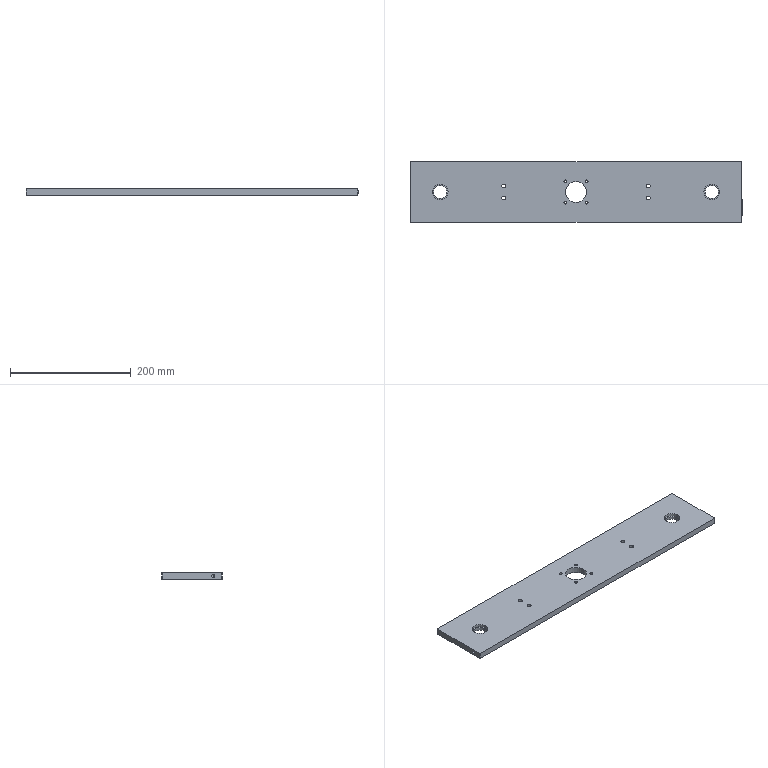Part | SolidWorks | features ICE 5, Extrusion 1, Fillet 1, HoleWzd 1, MirrorPattern 1 | 1 solid | 46 faces | box 550 x 100 x 10 mm | volume 528570 mm3 | cylinder 34 | plane 8 | cone 4 | commonest cylinder face diameters 4.5 x8 6.5 x8 2 x4 5 x4 22 x4 26 x4
STEP:
#1=CARTESIAN_POINT('',(257.,-35.,7.5));
#2=VERTEX_POINT('',#1);
#3=CARTESIAN_POINT('',(257.,-35.,2.5));
#4=VERTEX_POINT('',#3);
#5=CARTESIAN_POINT('',(257.,-35.,5.));
#6=DIRECTION('',(1.,0.,0.));
#7=DIRECTION('',(0.,0.,-1.));
#8=AXIS2_PLACEMENT_3D('',#5,#6,#7);
#9=CIRCLE('',#8,2.5);
#10=EDGE_CURVE('',#2,#4,#9,.T.);
#11=ORIENTED_EDGE('',*,*,#10,.F.);
#12=CARTESIAN_POINT('',(275.,-35.,7.5));
#13=VERTEX_POINT('',#12);
#14=CARTESIAN_POINT('',(275.,-35.,7.5));
#15=DIRECTION('',(1.,0.,0.));
#16=VECTOR('',#15,1000.);
#17=LINE('',#14,#16);
#18=EDGE_CURVE('',#2,#13,#17,.T.);
#19=ORIENTED_EDGE('',*,*,#18,.T.);
#20=CARTESIAN_POINT('',(275.,-35.,2.5));
#21=VERTEX_POINT('',#20);
#22=CARTESIAN_POINT('',(275.,-35.,5.));
#23=DIRECTION('',(1.,0.,0.));
#24=DIRECTION('',(0.,0.,-1.));
#25=AXIS2_PLACEMENT_3D('',#22,#23,#24);
#26=CIRCLE('',#25,2.5);
#27=EDGE_CURVE('',#13,#21,#26,.T.);
#28=ORIENTED_EDGE('',*,*,#27,.T.);
#29=CARTESIAN_POINT('',(275.,-35.,2.5));
#30=DIRECTION('',(1.,0.,0.));
#31=VECTOR('',#30,1000.);
#32=LINE('',#29,#31);
#33=EDGE_CURVE('',#4,#21,#32,.T.);
#34=ORIENTED_EDGE('',*,*,#33,.F.);
#35=EDGE_LOOP('',(#11,#19,#28,#34));
#36=FACE_OUTER_BOUND('',#35,.T.);
#37=CARTESIAN_POINT('',(275.,-35.,5.));
#38=DIRECTION('',(1.,0.,0.));
#39=DIRECTION('',(0.,0.,-1.));
#40=AXIS2_PLACEMENT_3D('',#37,#38,#39);
#41=CYLINDRICAL_SURFACE('',#40,2.5);
#42=ADVANCED_FACE('',(#36),#41,.F.);
#43=CARTESIAN_POINT('',(255.498,-35.,5.));
#44=VERTEX_POINT('',#43);
#45=CARTESIAN_POINT('',(257.,-35.,2.5));
#46=DIRECTION('',(0.515,0.,-0.8572));
#47=VECTOR('',#46,1000.);
#48=LINE('',#45,#47);
#49=EDGE_CURVE('',#44,#4,#48,.T.);
#50=ORIENTED_EDGE('',*,*,#49,.F.);
#51=CARTESIAN_POINT('',(257.,-35.,7.5));
#52=DIRECTION('',(0.515,0.,0.8572));
#53=VECTOR('',#52,1000.);
#54=LINE('',#51,#53);
#55=EDGE_CURVE('',#44,#2,#54,.T.);
#56=ORIENTED_EDGE('',*,*,#55,.T.);
#57=ORIENTED_EDGE('',*,*,#10,.T.);
#58=EDGE_LOOP('',(#50,#56,#57));
#59=FACE_OUTER_BOUND('',#58,.T.);
#60=CARTESIAN_POINT('',(257.,-35.,5.));
#61=DIRECTION('',(1.,0.,0.));
#62=DIRECTION('',(0.,0.,-1.));
#63=AXIS2_PLACEMENT_3D('',#60,#61,#62);
#64=CONICAL_SURFACE('',#63,2.5,1.03);
#65=ADVANCED_FACE('',(#59),#64,.F.);
#66=CARTESIAN_POINT('',(-257.,-35.,2.5));
#67=VERTEX_POINT('',#66);
#68=CARTESIAN_POINT('',(-257.,-35.,7.5));
#69=VERTEX_POINT('',#68);
#70=CARTESIAN_POINT('',(-257.,-35.,5.));
#71=DIRECTION('',(-1.,0.,0.));
#72=DIRECTION('',(0.,0.,1.));
#73=AXIS2_PLACEMENT_3D('',#70,#71,#72);
#74=CIRCLE('',#73,2.5);
#75=EDGE_CURVE('',#67,#69,#74,.T.);
#76=ORIENTED_EDGE('',*,*,#75,.F.);
#77=CARTESIAN_POINT('',(-275.,-35.,2.5));
#78=VERTEX_POINT('',#77);
#79=CARTESIAN_POINT('',(-275.,-35.,2.5));
#80=DIRECTION('',(-1.,0.,0.));
#81=VECTOR('',#80,1000.);
#82=LINE('',#79,#81);
#83=EDGE_CURVE('',#67,#78,#82,.T.);
#84=ORIENTED_EDGE('',*,*,#83,.T.);
#85=CARTESIAN_POINT('',(-275.,-35.,7.5));
#86=VERTEX_POINT('',#85);
#87=CARTESIAN_POINT('',(-275.,-35.,5.));
#88=DIRECTION('',(-1.,0.,0.));
#89=DIRECTION('',(0.,0.,1.));
#90=AXIS2_PLACEMENT_3D('',#87,#88,#89);
#91=CIRCLE('',#90,2.5);
#92=EDGE_CURVE('',#78,#86,#91,.T.);
#93=ORIENTED_EDGE('',*,*,#92,.T.);
#94=CARTESIAN_POINT('',(-275.,-35.,7.5));
#95=DIRECTION('',(-1.,0.,0.));
#96=VECTOR('',#95,1000.);
#97=LINE('',#94,#96);
#98=EDGE_CURVE('',#69,#86,#97,.T.);
#99=ORIENTED_EDGE('',*,*,#98,.F.);
#100=EDGE_LOOP('',(#76,#84,#93,#99));
#101=FACE_OUTER_BOUND('',#100,.T.);
#102=CARTESIAN_POINT('',(-275.,-35.,5.));
#103=DIRECTION('',(-1.,0.,0.));
#104=DIRECTION('',(0.,0.,1.));
#105=AXIS2_PLACEMENT_3D('',#102,#103,#104);
#106=CYLINDRICAL_SURFACE('',#105,2.5);
#107=ADVANCED_FACE('',(#101),#106,.F.);
#108=CARTESIAN_POINT('',(-255.498,-35.,5.));
#109=VERTEX_POINT('',#108);
#110=CARTESIAN_POINT('',(-257.,-35.,7.5));
#111=DIRECTION('',(-0.515,0.,0.8572));
#112=VECTOR('',#111,1000.);
#113=LINE('',#110,#112);
#114=EDGE_CURVE('',#109,#69,#113,.T.);
#115=ORIENTED_EDGE('',*,*,#114,.F.);
#116=CARTESIAN_POINT('',(-257.,-35.,2.5));
#117=DIRECTION('',(-0.515,0.,-0.8572));
#118=VECTOR('',#117,1000.);
#119=LINE('',#116,#118);
#120=EDGE_CURVE('',#109,#67,#119,.T.);
#121=ORIENTED_EDGE('',*,*,#120,.T.);
#122=ORIENTED_EDGE('',*,*,#75,.T.);
#123=EDGE_LOOP('',(#115,#121,#122));
#124=FACE_OUTER_BOUND('',#123,.T.);
#125=CARTESIAN_POINT('',(-257.,-35.,5.));
#126=DIRECTION('',(-1.,0.,0.));
#127=DIRECTION('',(0.,0.,1.));
#128=AXIS2_PLACEMENT_3D('',#125,#126,#127);
#129=CONICAL_SURFACE('',#128,2.5,1.03);
#130=ADVANCED_FACE('',(#124),#129,.F.);
#131=CARTESIAN_POINT('',(-123.25,10.,0.));
#132=VERTEX_POINT('',#131);
#133=CARTESIAN_POINT('',(-116.75,10.,0.));
#134=VERTEX_POINT('',#133);
#135=CARTESIAN_POINT('',(-120.,10.,0.));
#136=DIRECTION('',(0.,0.,1.));
#137=DIRECTION('',(1.,0.,0.));
#138=AXIS2_PLACEMENT_3D('',#135,#136,#137);
#139=CIRCLE('',#138,3.25);
#140=EDGE_CURVE('',#132,#134,#139,.T.);
#141=ORIENTED_EDGE('',*,*,#140,.F.);
#142=CARTESIAN_POINT('',(-123.25,10.,10.));
#143=VERTEX_POINT('',#142);
#144=CARTESIAN_POINT('',(-123.25,10.,0.));
#145=DIRECTION('',(0.,0.,1.));
#146=VECTOR('',#145,1000.);
#147=LINE('',#144,#146);
#148=EDGE_CURVE('',#132,#143,#147,.T.);
#149=ORIENTED_EDGE('',*,*,#148,.T.);
#150=CARTESIAN_POINT('',(-116.75,10.,10.));
#151=VERTEX_POINT('',#150);
#152=CARTESIAN_POINT('',(-120.,10.,10.));
#153=DIRECTION('',(0.,0.,1.));
#154=DIRECTION('',(1.,0.,0.));
#155=AXIS2_PLACEMENT_3D('',#152,#153,#154);
#156=CIRCLE('',#155,3.25);
#157=EDGE_CURVE('',#143,#151,#156,.T.);
#158=ORIENTED_EDGE('',*,*,#157,.T.);
#159=CARTESIAN_POINT('',(-116.75,10.,0.));
#160=DIRECTION('',(0.,0.,1.));
#161=VECTOR('',#160,1000.);
#162=LINE('',#159,#161);
#163=EDGE_CURVE('',#134,#151,#162,.T.);
#164=ORIENTED_EDGE('',*,*,#163,.F.);
#165=EDGE_LOOP('',(#141,#149,#158,#164));
#166=FACE_OUTER_BOUND('',#165,.T.);
#167=CARTESIAN_POINT('',(-120.,10.,0.));
#168=DIRECTION('',(0.,0.,1.));
#169=DIRECTION('',(1.,0.,0.));
#170=AXIS2_PLACEMENT_3D('',#167,#168,#169);
#171=CYLINDRICAL_SURFACE('',#170,3.25);
#172=ADVANCED_FACE('',(#166),#171,.F.);
#173=CARTESIAN_POINT('',(116.75,10.,0.));
#174=VERTEX_POINT('',#173);
#175=CARTESIAN_POINT('',(123.25,10.,0.));
#176=VERTEX_POINT('',#175);
#177=CARTESIAN_POINT('',(120.,10.,0.));
#178=DIRECTION('',(0.,0.,1.));
#179=DIRECTION('',(1.,0.,0.));
#180=AXIS2_PLACEMENT_3D('',#177,#178,#179);
#181=CIRCLE('',#180,3.25);
#182=EDGE_CURVE('',#174,#176,#181,.T.);
#183=ORIENTED_EDGE('',*,*,#182,.F.);
#184=CARTESIAN_POINT('',(116.75,10.,10.));
#185=VERTEX_POINT('',#184);
#186=CARTESIAN_POINT('',(116.75,10.,0.));
#187=DIRECTION('',(0.,0.,1.));
#188=VECTOR('',#187,1000.);
#189=LINE('',#186,#188);
#190=EDGE_CURVE('',#174,#185,#189,.T.);
#191=ORIENTED_EDGE('',*,*,#190,.T.);
#192=CARTESIAN_POINT('',(123.25,10.,10.));
#193=VERTEX_POINT('',#192);
#194=CARTESIAN_POINT('',(120.,10.,10.));
#195=DIRECTION('',(0.,0.,1.));
#196=DIRECTION('',(1.,0.,0.));
#197=AXIS2_PLACEMENT_3D('',#194,#195,#196);
#198=CIRCLE('',#197,3.25);
#199=EDGE_CURVE('',#185,#193,#198,.T.);
#200=ORIENTED_EDGE('',*,*,#199,.T.);
#201=CARTESIAN_POINT('',(123.25,10.,0.));
#202=DIRECTION('',(0.,0.,1.));
#203=VECTOR('',#202,1000.);
#204=LINE('',#201,#203);
#205=EDGE_CURVE('',#176,#193,#204,.T.);
#206=ORIENTED_EDGE('',*,*,#205,.F.);
#207=EDGE_LOOP('',(#183,#191,#200,#206));
#208=FACE_OUTER_BOUND('',#207,.T.);
#209=CARTESIAN_POINT('',(120.,10.,0.));
#210=DIRECTION('',(0.,0.,1.));
#211=DIRECTION('',(1.,0.,0.));
#212=AXIS2_PLACEMENT_3D('',#209,#210,#211);
#213=CYLINDRICAL_SURFACE('',#212,3.25);
#214=ADVANCED_FACE('',(#208),#213,.F.);
#215=CARTESIAN_POINT('',(116.75,-10.,0.));
#216=VERTEX_POINT('',#215);
#217=CARTESIAN_POINT('',(123.25,-10.,0.));
#218=VERTEX_POINT('',#217);
#219=CARTESIAN_POINT('',(120.,-10.,0.));
#220=DIRECTION('',(0.,0.,1.));
#221=DIRECTION('',(1.,0.,0.));
#222=AXIS2_PLACEMENT_3D('',#219,#220,#221);
#223=CIRCLE('',#222,3.25);
#224=EDGE_CURVE('',#216,#218,#223,.T.);
#225=ORIENTED_EDGE('',*,*,#224,.F.);
#226=CARTESIAN_POINT('',(116.75,-10.,10.));
#227=VERTEX_POINT('',#226);
#228=CARTESIAN_POINT('',(116.75,-10.,0.));
#229=DIRECTION('',(0.,0.,1.));
#230=VECTOR('',#229,1000.);
#231=LINE('',#228,#230);
#232=EDGE_CURVE('',#216,#227,#231,.T.);
#233=ORIENTED_EDGE('',*,*,#232,.T.);
#234=CARTESIAN_POINT('',(123.25,-10.,10.));
#235=VERTEX_POINT('',#234);
#236=CARTESIAN_POINT('',(120.,-10.,10.));
#237=DIRECTION('',(0.,0.,1.));
#238=DIRECTION('',(1.,0.,0.));
#239=AXIS2_PLACEMENT_3D('',#236,#237,#238);
#240=CIRCLE('',#239,3.25);
#241=EDGE_CURVE('',#227,#235,#240,.T.);
#242=ORIENTED_EDGE('',*,*,#241,.T.);
#243=CARTESIAN_POINT('',(123.25,-10.,0.));
#244=DIRECTION('',(0.,0.,1.));
#245=VECTOR('',#244,1000.);
#246=LINE('',#243,#245);
#247=EDGE_CURVE('',#218,#235,#246,.T.);
#248=ORIENTED_EDGE('',*,*,#247,.F.);
#249=EDGE_LOOP('',(#225,#233,#242,#248));
#250=FACE_OUTER_BOUND('',#249,.T.);
#251=CARTESIAN_POINT('',(120.,-10.,0.));
#252=DIRECTION('',(0.,0.,1.));
#253=DIRECTION('',(1.,0.,0.));
#254=AXIS2_PLACEMENT_3D('',#251,#252,#253);
#255=CYLINDRICAL_SURFACE('',#254,3.25);
#256=ADVANCED_FACE('',(#250),#255,.F.);
#257=CARTESIAN_POINT('',(-123.25,-10.,0.));
#258=VERTEX_POINT('',#257);
#259=CARTESIAN_POINT('',(-116.75,-10.,0.));
#260=VERTEX_POINT('',#259);
#261=CARTESIAN_POINT('',(-120.,-10.,0.));
#262=DIRECTION('',(0.,0.,1.));
#263=DIRECTION('',(1.,0.,0.));
#264=AXIS2_PLACEMENT_3D('',#261,#262,#263);
#265=CIRCLE('',#264,3.25);
#266=EDGE_CURVE('',#258,#260,#265,.T.);
#267=ORIENTED_EDGE('',*,*,#266,.F.);
#268=CARTESIAN_POINT('',(-123.25,-10.,10.));
#269=VERTEX_POINT('',#268);
#270=CARTESIAN_POINT('',(-123.25,-10.,0.));
#271=DIRECTION('',(0.,0.,1.));
#272=VECTOR('',#271,1000.);
#273=LINE('',#270,#272);
#274=EDGE_CURVE('',#258,#269,#273,.T.);
#275=ORIENTED_EDGE('',*,*,#274,.T.);
#276=CARTESIAN_POINT('',(-116.75,-10.,10.));
#277=VERTEX_POINT('',#276);
#278=CARTESIAN_POINT('',(-120.,-10.,10.));
#279=DIRECTION('',(0.,0.,1.));
#280=DIRECTION('',(1.,0.,0.));
#281=AXIS2_PLACEMENT_3D('',#278,#279,#280);
#282=CIRCLE('',#281,3.25);
#283=EDGE_CURVE('',#269,#277,#282,.T.);
#284=ORIENTED_EDGE('',*,*,#283,.T.);
#285=CARTESIAN_POINT('',(-116.75,-10.,0.));
#286=DIRECTION('',(0.,0.,1.));
#287=VECTOR('',#286,1000.);
#288=LINE('',#285,#287);
#289=EDGE_CURVE('',#260,#277,#288,.T.);
#290=ORIENTED_EDGE('',*,*,#289,.F.);
#291=EDGE_LOOP('',(#267,#275,#284,#290));
#292=FACE_OUTER_BOUND('',#291,.T.);
#293=CARTESIAN_POINT('',(-120.,-10.,0.));
#294=DIRECTION('',(0.,0.,1.));
#295=DIRECTION('',(1.,0.,0.));
#296=AXIS2_PLACEMENT_3D('',#293,#294,#295);
#297=CYLINDRICAL_SURFACE('',#296,3.25);
#298=ADVANCED_FACE('',(#292),#297,.F.);
#299=CARTESIAN_POINT('',(-19.928,-17.678,0.));
#300=VERTEX_POINT('',#299);
#301=CARTESIAN_POINT('',(-15.428,-17.678,0.));
#302=VERTEX_POINT('',#301);
#303=CARTESIAN_POINT('',(-17.678,-17.678,0.));
#304=DIRECTION('',(0.,0.,1.));
#305=DIRECTION('',(1.,0.,0.));
#306=AXIS2_PLACEMENT_3D('',#303,#304,#305);
#307=CIRCLE('',#306,2.25);
#308=EDGE_CURVE('',#300,#302,#307,.T.);
#309=ORIENTED_EDGE('',*,*,#308,.F.);
#310=CARTESIAN_POINT('',(-19.928,-17.678,10.));
#311=VERTEX_POINT('',#310);
#312=CARTESIAN_POINT('',(-19.928,-17.678,0.));
#313=DIRECTION('',(0.,0.,1.));
#314=VECTOR('',#313,1000.);
#315=LINE('',#312,#314);
#316=EDGE_CURVE('',#300,#311,#315,.T.);
#317=ORIENTED_EDGE('',*,*,#316,.T.);
#318=CARTESIAN_POINT('',(-15.428,-17.678,10.));
#319=VERTEX_POINT('',#318);
#320=CARTESIAN_POINT('',(-17.678,-17.678,10.));
#321=DIRECTION('',(0.,0.,1.));
#322=DIRECTION('',(1.,0.,0.));
#323=AXIS2_PLACEMENT_3D('',#320,#321,#322);
#324=CIRCLE('',#323,2.25);
#325=EDGE_CURVE('',#311,#319,#324,.T.);
#326=ORIENTED_EDGE('',*,*,#325,.T.);
#327=CARTESIAN_POINT('',(-15.428,-17.678,0.));
#328=DIRECTION('',(0.,0.,1.));
#329=VECTOR('',#328,1000.);
#330=LINE('',#327,#329);
#331=EDGE_CURVE('',#302,#319,#330,.T.);
#332=ORIENTED_EDGE('',*,*,#331,.F.);
#333=EDGE_LOOP('',(#309,#317,#326,#332));
#334=FACE_OUTER_BOUND('',#333,.T.);
#335=CARTESIAN_POINT('',(-17.678,-17.678,0.));
#336=DIRECTION('',(0.,0.,1.));
#337=DIRECTION('',(1.,0.,0.));
#338=AXIS2_PLACEMENT_3D('',#335,#336,#337);
#339=CYLINDRICAL_SURFACE('',#338,2.25);
#340=ADVANCED_FACE('',(#334),#339,.F.);
#341=CARTESIAN_POINT('',(15.428,-17.678,0.));
#342=VERTEX_POINT('',#341);
#343=CARTESIAN_POINT('',(19.928,-17.678,0.));
#344=VERTEX_POINT('',#343);
#345=CARTESIAN_POINT('',(17.678,-17.678,0.));
#346=DIRECTION('',(0.,0.,1.));
#347=DIRECTION('',(1.,0.,0.));
#348=AXIS2_PLACEMENT_3D('',#345,#346,#347);
#349=CIRCLE('',#348,2.25);
#350=EDGE_CURVE('',#342,#344,#349,.T.);
#351=ORIENTED_EDGE('',*,*,#350,.F.);
#352=CARTESIAN_POINT('',(15.428,-17.678,10.));
#353=VERTEX_POINT('',#352);
#354=CARTESIAN_POINT('',(15.428,-17.678,0.));
#355=DIRECTION('',(0.,0.,1.));
#356=VECTOR('',#355,1000.);
#357=LINE('',#354,#356);
#358=EDGE_CURVE('',#342,#353,#357,.T.);
#359=ORIENTED_EDGE('',*,*,#358,.T.);
#360=CARTESIAN_POINT('',(19.928,-17.678,10.));
#361=VERTEX_POINT('',#360);
#362=CARTESIAN_POINT('',(17.678,-17.678,10.));
#363=DIRECTION('',(0.,0.,1.));
#364=DIRECTION('',(1.,0.,0.));
#365=AXIS2_PLACEMENT_3D('',#362,#363,#364);
#366=CIRCLE('',#365,2.25);
#367=EDGE_CURVE('',#353,#361,#366,.T.);
#368=ORIENTED_EDGE('',*,*,#367,.T.);
#369=CARTESIAN_POINT('',(19.928,-17.678,0.));
#370=DIRECTION('',(0.,0.,1.));
#371=VECTOR('',#370,1000.);
#372=LINE('',#369,#371);
#373=EDGE_CURVE('',#344,#361,#372,.T.);
#374=ORIENTED_EDGE('',*,*,#373,.F.);
#375=EDGE_LOOP('',(#351,#359,#368,#374));
#376=FACE_OUTER_BOUND('',#375,.T.);
#377=CARTESIAN_POINT('',(17.678,-17.678,0.));
#378=DIRECTION('',(0.,0.,1.));
#379=DIRECTION('',(1.,0.,0.));
#380=AXIS2_PLACEMENT_3D('',#377,#378,#379);
#381=CYLINDRICAL_SURFACE('',#380,2.25);
#382=ADVANCED_FACE('',(#376),#381,.F.);
#383=CARTESIAN_POINT('',(15.428,17.678,0.));
#384=VERTEX_POINT('',#383);
#385=CARTESIAN_POINT('',(19.928,17.678,0.));
#386=VERTEX_POINT('',#385);
#387=CARTESIAN_POINT('',(17.678,17.678,0.));
#388=DIRECTION('',(0.,0.,1.));
#389=DIRECTION('',(1.,0.,0.));
#390=AXIS2_PLACEMENT_3D('',#387,#388,#389);
#391=CIRCLE('',#390,2.25);
#392=EDGE_CURVE('',#384,#386,#391,.T.);
#393=ORIENTED_EDGE('',*,*,#392,.F.);
#394=CARTESIAN_POINT('',(15.428,17.678,10.));
#395=VERTEX_POINT('',#394);
#396=CARTESIAN_POINT('',(15.428,17.678,0.));
#397=DIRECTION('',(0.,0.,1.));
#398=VECTOR('',#397,1000.);
#399=LINE('',#396,#398);
#400=EDGE_CURVE('',#384,#395,#399,.T.);
#401=ORIENTED_EDGE('',*,*,#400,.T.);
#402=CARTESIAN_POINT('',(19.928,17.678,10.));
#403=VERTEX_POINT('',#402);
#404=CARTESIAN_POINT('',(17.678,17.678,10.));
#405=DIRECTION('',(0.,0.,1.));
#406=DIRECTION('',(1.,0.,0.));
#407=AXIS2_PLACEMENT_3D('',#404,#405,#406);
#408=CIRCLE('',#407,2.25);
#409=EDGE_CURVE('',#395,#403,#408,.T.);
#410=ORIENTED_EDGE('',*,*,#409,.T.);
#411=CARTESIAN_POINT('',(19.928,17.678,0.));
#412=DIRECTION('',(0.,0.,1.));
#413=VECTOR('',#412,1000.);
#414=LINE('',#411,#413);
#415=EDGE_CURVE('',#386,#403,#414,.T.);
#416=ORIENTED_EDGE('',*,*,#415,.F.);
#417=EDGE_LOOP('',(#393,#401,#410,#416));
#418=FACE_OUTER_BOUND('',#417,.T.);
#419=CARTESIAN_POINT('',(17.678,17.678,0.));
#420=DIRECTION('',(0.,0.,1.));
#421=DIRECTION('',(1.,0.,0.));
#422=AXIS2_PLACEMENT_3D('',#419,#420,#421);
#423=CYLINDRICAL_SURFACE('',#422,2.25);
#424=ADVANCED_FACE('',(#418),#423,.F.);
#425=CARTESIAN_POINT('',(-19.928,17.678,0.));
#426=VERTEX_POINT('',#425);
#427=CARTESIAN_POINT('',(-15.428,17.678,0.));
#428=VERTEX_POINT('',#427);
#429=CARTESIAN_POINT('',(-17.678,17.678,0.));
#430=DIRECTION('',(0.,0.,1.));
#431=DIRECTION('',(1.,0.,0.));
#432=AXIS2_PLACEMENT_3D('',#429,#430,#431);
#433=CIRCLE('',#432,2.25);
#434=EDGE_CURVE('',#426,#428,#433,.T.);
#435=ORIENTED_EDGE('',*,*,#434,.F.);
#436=CARTESIAN_POINT('',(-19.928,17.678,10.));
#437=VERTEX_POINT('',#436);
#438=CARTESIAN_POINT('',(-19.928,17.678,0.));
#439=DIRECTION('',(0.,0.,1.));
#440=VECTOR('',#439,1000.);
#441=LINE('',#438,#440);
#442=EDGE_CURVE('',#426,#437,#441,.T.);
#443=ORIENTED_EDGE('',*,*,#442,.T.);
#444=CARTESIAN_POINT('',(-15.428,17.678,10.));
#445=VERTEX_POINT('',#444);
#446=CARTESIAN_POINT('',(-17.678,17.678,10.));
#447=DIRECTION('',(0.,0.,1.));
#448=DIRECTION('',(1.,0.,0.));
#449=AXIS2_PLACEMENT_3D('',#446,#447,#448);
#450=CIRCLE('',#449,2.25);
#451=EDGE_CURVE('',#437,#445,#450,.T.);
#452=ORIENTED_EDGE('',*,*,#451,.T.);
#453=CARTESIAN_POINT('',(-15.428,17.678,0.));
#454=DIRECTION('',(0.,0.,1.));
#455=VECTOR('',#454,1000.);
#456=LINE('',#453,#455);
#457=EDGE_CURVE('',#428,#445,#456,.T.);
#458=ORIENTED_EDGE('',*,*,#457,.F.);
#459=EDGE_LOOP('',(#435,#443,#452,#458));
#460=FACE_OUTER_BOUND('',#459,.T.);
#461=CARTESIAN_POINT('',(-17.678,17.678,0.));
#462=DIRECTION('',(0.,0.,1.));
#463=DIRECTION('',(1.,0.,0.));
#464=AXIS2_PLACEMENT_3D('',#461,#462,#463);
#465=CYLINDRICAL_SURFACE('',#464,2.25);
#466=ADVANCED_FACE('',(#460),#465,.F.);
#467=CARTESIAN_POINT('',(-17.5,0.,0.));
#468=VERTEX_POINT('',#467);
#469=CARTESIAN_POINT('',(17.5,0.,0.));
#470=VERTEX_POINT('',#469);
#471=CARTESIAN_POINT('',(0.,0.,0.));
#472=DIRECTION('',(0.,0.,1.));
#473=DIRECTION('',(1.,0.,0.));
#474=AXIS2_PLACEMENT_3D('',#471,#472,#473);
#475=CIRCLE('',#474,17.5);
#476=EDGE_CURVE('',#468,#470,#475,.T.);
#477=ORIENTED_EDGE('',*,*,#476,.F.);
#478=CARTESIAN_POINT('',(-17.5,0.,10.));
#479=VERTEX_POINT('',#478);
#480=CARTESIAN_POINT('',(-17.5,0.,0.));
#481=DIRECTION('',(0.,0.,1.));
#482=VECTOR('',#481,1000.);
#483=LINE('',#480,#482);
#484=EDGE_CURVE('',#468,#479,#483,.T.);
#485=ORIENTED_EDGE('',*,*,#484,.T.);
#486=CARTESIAN_POINT('',(17.5,0.,10.));
#487=VERTEX_POINT('',#486);
#488=CARTESIAN_POINT('',(0.,0.,10.));
#489=DIRECTION('',(0.,0.,1.));
#490=DIRECTION('',(1.,0.,0.));
#491=AXIS2_PLACEMENT_3D('',#488,#489,#490);
#492=CIRCLE('',#491,17.5);
#493=EDGE_CURVE('',#479,#487,#492,.T.);
#494=ORIENTED_EDGE('',*,*,#493,.T.);
#495=CARTESIAN_POINT('',(17.5,0.,0.));
#496=DIRECTION('',(0.,0.,1.));
#497=VECTOR('',#496,1000.);
#498=LINE('',#495,#497);
#499=EDGE_CURVE('',#470,#487,#498,.T.);
#500=ORIENTED_EDGE('',*,*,#499,.F.);
#501=EDGE_LOOP('',(#477,#485,#494,#500));
#502=FACE_OUTER_BOUND('',#501,.T.);
#503=CARTESIAN_POINT('',(0.,0.,0.));
#504=DIRECTION('',(0.,0.,1.));
#505=DIRECTION('',(1.,0.,0.));
#506=AXIS2_PLACEMENT_3D('',#503,#504,#505);
#507=CYLINDRICAL_SURFACE('',#506,17.5);
#508=ADVANCED_FACE('',(#502),#507,.F.);
#509=CARTESIAN_POINT('',(214.,0.,0.));
#510=VERTEX_POINT('',#509);
#511=CARTESIAN_POINT('',(236.,0.,0.));
#512=VERTEX_POINT('',#511);
#513=CARTESIAN_POINT('',(225.,0.,0.));
#514=DIRECTION('',(0.,0.,1.));
#515=DIRECTION('',(1.,0.,0.));
#516=AXIS2_PLACEMENT_3D('',#513,#514,#515);
#517=CIRCLE('',#516,11.);
#518=EDGE_CURVE('',#510,#512,#517,.T.);
#519=ORIENTED_EDGE('',*,*,#518,.F.);
#520=CARTESIAN_POINT('',(214.,0.,5.));
#521=VERTEX_POINT('',#520);
#522=CARTESIAN_POINT('',(214.,0.,0.));
#523=DIRECTION('',(0.,0.,1.));
#524=VECTOR('',#523,1000.);
#525=LINE('',#522,#524);
#526=EDGE_CURVE('',#510,#521,#525,.T.);
#527=ORIENTED_EDGE('',*,*,#526,.T.);
#528=CARTESIAN_POINT('',(236.,0.,5.));
#529=VERTEX_POINT('',#528);
#530=CARTESIAN_POINT('',(225.,0.,5.));
#531=DIRECTION('',(0.,0.,1.));
#532=DIRECTION('',(1.,0.,0.));
#533=AXIS2_PLACEMENT_3D('',#530,#531,#532);
#534=CIRCLE('',#533,11.);
#535=EDGE_CURVE('',#521,#529,#534,.T.);
#536=ORIENTED_EDGE('',*,*,#535,.T.);
#537=CARTESIAN_POINT('',(236.,0.,0.));
#538=DIRECTION('',(0.,0.,1.));
#539=VECTOR('',#538,1000.);
#540=LINE('',#537,#539);
#541=EDGE_CURVE('',#512,#529,#540,.T.);
#542=ORIENTED_EDGE('',*,*,#541,.F.);
#543=EDGE_LOOP('',(#519,#527,#536,#542));
#544=FACE_OUTER_BOUND('',#543,.T.);
#545=CARTESIAN_POINT('',(225.,0.,0.));
#546=DIRECTION('',(0.,0.,1.));
#547=DIRECTION('',(1.,0.,0.));
#548=AXIS2_PLACEMENT_3D('',#545,#546,#547);
#549=CYLINDRICAL_SURFACE('',#548,11.);
#550=ADVANCED_FACE('',(#544),#549,.F.);
#551=CARTESIAN_POINT('',(-236.,0.,0.));
#552=VERTEX_POINT('',#551);
#553=CARTESIAN_POINT('',(-214.,0.,0.));
#554=VERTEX_POINT('',#553);
#555=CARTESIAN_POINT('',(-225.,0.,0.));
#556=DIRECTION('',(0.,0.,1.));
#557=DIRECTION('',(-1.,0.,0.));
#558=AXIS2_PLACEMENT_3D('',#555,#556,#557);
#559=CIRCLE('',#558,11.);
#560=EDGE_CURVE('',#552,#554,#559,.T.);
#561=ORIENTED_EDGE('',*,*,#560,.F.);
#562=CARTESIAN_POINT('',(-236.,0.,5.));
#563=VERTEX_POINT('',#562);
#564=CARTESIAN_POINT('',(-236.,0.,0.));
#565=DIRECTION('',(0.,0.,1.));
#566=VECTOR('',#565,1000.);
#567=LINE('',#564,#566);
#568=EDGE_CURVE('',#552,#563,#567,.T.);
#569=ORIENTED_EDGE('',*,*,#568,.T.);
#570=CARTESIAN_POINT('',(-214.,0.,5.));
#571=VERTEX_POINT('',#570);
#572=CARTESIAN_POINT('',(-225.,0.,5.));
#573=DIRECTION('',(0.,0.,1.));
#574=DIRECTION('',(-1.,0.,0.));
#575=AXIS2_PLACEMENT_3D('',#572,#573,#574);
#576=CIRCLE('',#575,11.);
#577=EDGE_CURVE('',#563,#571,#576,.T.);
#578=ORIENTED_EDGE('',*,*,#577,.T.);
#579=CARTESIAN_POINT('',(-214.,0.,0.));
#580=DIRECTION('',(0.,0.,1.));
#581=VECTOR('',#580,1000.);
#582=LINE('',#579,#581);
#583=EDGE_CURVE('',#554,#571,#582,.T.);
#584=ORIENTED_EDGE('',*,*,#583,.F.);
#585=EDGE_LOOP('',(#561,#569,#578,#584));
#586=FACE_OUTER_BOUND('',#585,.T.);
#587=CARTESIAN_POINT('',(-225.,0.,0.));
#588=DIRECTION('',(0.,0.,1.));
#589=DIRECTION('',(1.,0.,0.));
#590=AXIS2_PLACEMENT_3D('',#587,#588,#589);
#591=CYLINDRICAL_SURFACE('',#590,11.);
#592=ADVANCED_FACE('',(#586),#591,.F.);
#593=CARTESIAN_POINT('',(212.,0.,5.));
#594=VERTEX_POINT('',#593);
#595=CARTESIAN_POINT('',(238.,0.,5.));
#596=VERTEX_POINT('',#595);
#597=CARTESIAN_POINT('',(225.,0.,5.));
#598=DIRECTION('',(0.,0.,1.));
#599=DIRECTION('',(1.,0.,0.));
#600=AXIS2_PLACEMENT_3D('',#597,#598,#599);
#601=CIRCLE('',#600,13.);
#602=EDGE_CURVE('',#594,#596,#601,.T.);
#603=ORIENTED_EDGE('',*,*,#602,.F.);
#604=CARTESIAN_POINT('',(212.,0.,10.));
#605=VERTEX_POINT('',#604);
#606=CARTESIAN_POINT('',(212.,0.,5.));
#607=DIRECTION('',(0.,0.,1.));
#608=VECTOR('',#607,1000.);
#609=LINE('',#606,#608);
#610=EDGE_CURVE('',#594,#605,#609,.T.);
#611=ORIENTED_EDGE('',*,*,#610,.T.);
#612=CARTESIAN_POINT('',(238.,0.,10.));
#613=VERTEX_POINT('',#612);
#614=CARTESIAN_POINT('',(225.,0.,10.));
#615=DIRECTION('',(0.,0.,1.));
#616=DIRECTION('',(1.,0.,0.));
#617=AXIS2_PLACEMENT_3D('',#614,#615,#616);
#618=CIRCLE('',#617,13.);
#619=EDGE_CURVE('',#605,#613,#618,.T.);
#620=ORIENTED_EDGE('',*,*,#619,.T.);
#621=CARTESIAN_POINT('',(238.,0.,5.));
#622=DIRECTION('',(0.,0.,1.));
#623=VECTOR('',#622,1000.);
#624=LINE('',#621,#623);
#625=EDGE_CURVE('',#596,#613,#624,.T.);
#626=ORIENTED_EDGE('',*,*,#625,.F.);
#627=EDGE_LOOP('',(#603,#611,#620,#626));
#628=FACE_OUTER_BOUND('',#627,.T.);
#629=CARTESIAN_POINT('',(225.,0.,5.));
#630=DIRECTION('',(0.,0.,1.));
#631=DIRECTION('',(1.,0.,0.));
#632=AXIS2_PLACEMENT_3D('',#629,#630,#631);
#633=CYLINDRICAL_SURFACE('',#632,13.);
#634=ADVANCED_FACE('',(#628),#633,.F.);
#635=CARTESIAN_POINT('',(-238.,0.,5.));
#636=VERTEX_POINT('',#635);
#637=CARTESIAN_POINT('',(-212.,0.,5.));
#638=VERTEX_POINT('',#637);
#639=CARTESIAN_POINT('',(-225.,0.,5.));
#640=DIRECTION('',(0.,0.,1.));
#641=DIRECTION('',(-1.,0.,0.));
#642=AXIS2_PLACEMENT_3D('',#639,#640,#641);
#643=CIRCLE('',#642,13.);
#644=EDGE_CURVE('',#636,#638,#643,.T.);
#645=ORIENTED_EDGE('',*,*,#644,.F.);
#646=CARTESIAN_POINT('',(-238.,0.,10.));
#647=VERTEX_POINT('',#646);
#648=CARTESIAN_POINT('',(-238.,0.,5.));
#649=DIRECTION('',(0.,0.,1.));
#650=VECTOR('',#649,1000.);
#651=LINE('',#648,#650);
#652=EDGE_CURVE('',#636,#647,#651,.T.);
#653=ORIENTED_EDGE('',*,*,#652,.T.);
#654=CARTESIAN_POINT('',(-212.,0.,10.));
#655=VERTEX_POINT('',#654);
#656=CARTESIAN_POINT('',(-225.,0.,10.));
#657=DIRECTION('',(0.,0.,1.));
#658=DIRECTION('',(-1.,0.,0.));
#659=AXIS2_PLACEMENT_3D('',#656,#657,#658);
#660=CIRCLE('',#659,13.);
#661=EDGE_CURVE('',#647,#655,#660,.T.);
#662=ORIENTED_EDGE('',*,*,#661,.T.);
#663=CARTESIAN_POINT('',(-212.,0.,5.));
#664=DIRECTION('',(0.,0.,1.));
#665=VECTOR('',#664,1000.);
#666=LINE('',#663,#665);
#667=EDGE_CURVE('',#638,#655,#666,.T.);
#668=ORIENTED_EDGE('',*,*,#667,.F.);
#669=EDGE_LOOP('',(#645,#653,#662,#668));
#670=FACE_OUTER_BOUND('',#669,.T.);
#671=CARTESIAN_POINT('',(-225.,0.,5.));
#672=DIRECTION('',(0.,0.,1.));
#673=DIRECTION('',(1.,0.,0.));
#674=AXIS2_PLACEMENT_3D('',#671,#672,#673);
#675=CYLINDRICAL_SURFACE('',#674,13.);
#676=ADVANCED_FACE('',(#670),#675,.F.);
#677=CARTESIAN_POINT('',(-275.,-35.,5.));
#678=DIRECTION('',(-1.,0.,0.));
#679=DIRECTION('',(0.,0.,1.));
#680=AXIS2_PLACEMENT_3D('',#677,#678,#679);
#681=CIRCLE('',#680,2.5);
#682=EDGE_CURVE('',#86,#78,#681,.T.);
#683=ORIENTED_EDGE('',*,*,#682,.F.);
#684=ORIENTED_EDGE('',*,*,#92,.F.);
#685=EDGE_LOOP('',(#683,#684));
#686=FACE_BOUND('',#685,.T.);
#687=CARTESIAN_POINT('',(-275.,49.,0.));
#688=VERTEX_POINT('',#687);
#689=CARTESIAN_POINT('',(-275.,-49.,0.));
#690=VERTEX_POINT('',#689);
#691=CARTESIAN_POINT('',(-275.,-50.,0.));
#692=DIRECTION('',(0.,-1.,0.));
#693=VECTOR('',#692,1000.);
#694=LINE('',#691,#693);
#695=EDGE_CURVE('',#688,#690,#694,.T.);
#696=ORIENTED_EDGE('',*,*,#695,.T.);
#697=CARTESIAN_POINT('',(-275.,-49.,10.));
#698=VERTEX_POINT('',#697);
#699=CARTESIAN_POINT('',(-275.,-49.,10.));
#700=DIRECTION('',(0.,0.,1.));
#701=VECTOR('',#700,1000.);
#702=LINE('',#699,#701);
#703=EDGE_CURVE('',#690,#698,#702,.T.);
#704=ORIENTED_EDGE('',*,*,#703,.T.);
#705=CARTESIAN_POINT('',(-275.,49.,10.));
#706=VERTEX_POINT('',#705);
#707=CARTESIAN_POINT('',(-275.,-50.,10.));
#708=DIRECTION('',(0.,-1.,0.));
#709=VECTOR('',#708,1000.);
#710=LINE('',#707,#709);
#711=EDGE_CURVE('',#706,#698,#710,.T.);
#712=ORIENTED_EDGE('',*,*,#711,.F.);
#713=CARTESIAN_POINT('',(-275.,49.,10.));
#714=DIRECTION('',(0.,0.,-1.));
#715=VECTOR('',#714,1000.);
#716=LINE('',#713,#715);
#717=EDGE_CURVE('',#706,#688,#716,.T.);
#718=ORIENTED_EDGE('',*,*,#717,.T.);
#719=EDGE_LOOP('',(#696,#704,#712,#718));
#720=FACE_OUTER_BOUND('',#719,.T.);
#721=CARTESIAN_POINT('',(-275.,-50.,10.));
#722=DIRECTION('',(1.,0.,0.));
#723=DIRECTION('',(0.,0.,-1.));
#724=AXIS2_PLACEMENT_3D('',#721,#722,#723);
#725=PLANE('',#724);
#726=ADVANCED_FACE('',(#686,#720),#725,.F.);
#727=CARTESIAN_POINT('',(-274.,-50.,10.));
#728=VERTEX_POINT('',#727);
#729=CARTESIAN_POINT('',(274.,-50.,10.));
#730=VERTEX_POINT('',#729);
#731=CARTESIAN_POINT('',(275.,-50.,10.));
#732=DIRECTION('',(1.,0.,0.));
#733=VECTOR('',#732,1000.);
#734=LINE('',#731,#733);
#735=EDGE_CURVE('',#728,#730,#734,.T.);
#736=ORIENTED_EDGE('',*,*,#735,.F.);
#737=CARTESIAN_POINT('',(-274.,-50.,0.));
#738=VERTEX_POINT('',#737);
#739=CARTESIAN_POINT('',(-274.,-50.,10.));
#740=DIRECTION('',(0.,0.,-1.));
#741=VECTOR('',#740,1000.);
#742=LINE('',#739,#741);
#743=EDGE_CURVE('',#728,#738,#742,.T.);
#744=ORIENTED_EDGE('',*,*,#743,.T.);
#745=CARTESIAN_POINT('',(274.,-50.,0.));
#746=VERTEX_POINT('',#745);
#747=CARTESIAN_POINT('',(275.,-50.,0.));
#748=DIRECTION('',(1.,0.,0.));
#749=VECTOR('',#748,1000.);
#750=LINE('',#747,#749);
#751=EDGE_CURVE('',#738,#746,#750,.T.);
#752=ORIENTED_EDGE('',*,*,#751,.T.);
#753=CARTESIAN_POINT('',(274.,-50.,10.));
#754=DIRECTION('',(0.,0.,1.));
#755=VECTOR('',#754,1000.);
#756=LINE('',#753,#755);
#757=EDGE_CURVE('',#746,#730,#756,.T.);
#758=ORIENTED_EDGE('',*,*,#757,.T.);
#759=EDGE_LOOP('',(#736,#744,#752,#758));
#760=FACE_OUTER_BOUND('',#759,.T.);
#761=CARTESIAN_POINT('',(275.,-50.,10.));
#762=DIRECTION('',(0.,1.,0.));
#763=DIRECTION('',(-1.,0.,0.));
#764=AXIS2_PLACEMENT_3D('',#761,#762,#763);
#765=PLANE('',#764);
#766=ADVANCED_FACE('',(#760),#765,.F.);
#767=CARTESIAN_POINT('',(275.,-35.,5.));
#768=DIRECTION('',(1.,0.,0.));
#769=DIRECTION('',(0.,0.,-1.));
#770=AXIS2_PLACEMENT_3D('',#767,#768,#769);
#771=CIRCLE('',#770,2.5);
#772=EDGE_CURVE('',#21,#13,#771,.T.);
#773=ORIENTED_EDGE('',*,*,#772,.F.);
#774=ORIENTED_EDGE('',*,*,#27,.F.);
#775=EDGE_LOOP('',(#773,#774));
#776=FACE_BOUND('',#775,.T.);
#777=CARTESIAN_POINT('',(275.,-49.,10.));
#778=VERTEX_POINT('',#777);
#779=CARTESIAN_POINT('',(275.,49.,10.));
#780=VERTEX_POINT('',#779);
#781=CARTESIAN_POINT('',(275.,-50.,10.));
#782=DIRECTION('',(0.,1.,0.));
#783=VECTOR('',#782,1000.);
#784=LINE('',#781,#783);
#785=EDGE_CURVE('',#778,#780,#784,.T.);
#786=ORIENTED_EDGE('',*,*,#785,.F.);
#787=CARTESIAN_POINT('',(275.,-49.,0.));
#788=VERTEX_POINT('',#787);
#789=CARTESIAN_POINT('',(275.,-49.,10.));
#790=DIRECTION('',(0.,0.,-1.));
#791=VECTOR('',#790,1000.);
#792=LINE('',#789,#791);
#793=EDGE_CURVE('',#778,#788,#792,.T.);
#794=ORIENTED_EDGE('',*,*,#793,.T.);
#795=CARTESIAN_POINT('',(275.,49.,0.));
#796=VERTEX_POINT('',#795);
#797=CARTESIAN_POINT('',(275.,-50.,0.));
#798=DIRECTION('',(0.,1.,0.));
#799=VECTOR('',#798,1000.);
#800=LINE('',#797,#799);
#801=EDGE_CURVE('',#788,#796,#800,.T.);
#802=ORIENTED_EDGE('',*,*,#801,.T.);
#803=CARTESIAN_POINT('',(275.,49.,10.));
#804=DIRECTION('',(0.,0.,1.));
#805=VECTOR('',#804,1000.);
#806=LINE('',#803,#805);
#807=EDGE_CURVE('',#796,#780,#806,.T.);
#808=ORIENTED_EDGE('',*,*,#807,.T.);
#809=EDGE_LOOP('',(#786,#794,#802,#808));
#810=FACE_OUTER_BOUND('',#809,.T.);
#811=CARTESIAN_POINT('',(275.,-50.,10.));
#812=DIRECTION('',(-1.,0.,0.));
#813=DIRECTION('',(0.,0.,1.));
#814=AXIS2_PLACEMENT_3D('',#811,#812,#813);
#815=PLANE('',#814);
#816=ADVANCED_FACE('',(#776,#810),#815,.F.);
#817=CARTESIAN_POINT('',(274.,50.,0.));
#818=VERTEX_POINT('',#817);
#819=CARTESIAN_POINT('',(-274.,50.,0.));
#820=VERTEX_POINT('',#819);
#821=CARTESIAN_POINT('',(275.,50.,0.));
#822=DIRECTION('',(-1.,0.,0.));
#823=VECTOR('',#822,1000.);
#824=LINE('',#821,#823);
#825=EDGE_CURVE('',#818,#820,#824,.T.);
#826=ORIENTED_EDGE('',*,*,#825,.T.);
#827=CARTESIAN_POINT('',(-274.,50.,10.));
#828=VERTEX_POINT('',#827);
#829=CARTESIAN_POINT('',(-274.,50.,10.));
#830=DIRECTION('',(0.,0.,1.));
#831=VECTOR('',#830,1000.);
#832=LINE('',#829,#831);
#833=EDGE_CURVE('',#820,#828,#832,.T.);
#834=ORIENTED_EDGE('',*,*,#833,.T.);
#835=CARTESIAN_POINT('',(274.,50.,10.));
#836=VERTEX_POINT('',#835);
#837=CARTESIAN_POINT('',(275.,50.,10.));
#838=DIRECTION('',(-1.,0.,0.));
#839=VECTOR('',#838,1000.);
#840=LINE('',#837,#839);
#841=EDGE_CURVE('',#836,#828,#840,.T.);
#842=ORIENTED_EDGE('',*,*,#841,.F.);
#843=CARTESIAN_POINT('',(274.,50.,10.));
#844=DIRECTION('',(0.,0.,-1.));
#845=VECTOR('',#844,1000.);
#846=LINE('',#843,#845);
#847=EDGE_CURVE('',#836,#818,#846,.T.);
#848=ORIENTED_EDGE('',*,*,#847,.T.);
#849=EDGE_LOOP('',(#826,#834,#842,#848));
#850=FACE_OUTER_BOUND('',#849,.T.);
#851=CARTESIAN_POINT('',(275.,50.,10.));
#852=DIRECTION('',(0.,-1.,0.));
#853=DIRECTION('',(1.,0.,0.));
#854=AXIS2_PLACEMENT_3D('',#851,#852,#853);
#855=PLANE('',#854);
#856=ADVANCED_FACE('',(#850),#855,.F.);
#857=CARTESIAN_POINT('',(-120.,10.,10.));
#858=DIRECTION('',(0.,0.,1.));
#859=DIRECTION('',(1.,0.,0.));
#860=AXIS2_PLACEMENT_3D('',#857,#858,#859);
#861=CIRCLE('',#860,3.25);
#862=EDGE_CURVE('',#151,#143,#861,.T.);
#863=ORIENTED_EDGE('',*,*,#862,.F.);
#864=ORIENTED_EDGE('',*,*,#157,.F.);
#865=EDGE_LOOP('',(#863,#864));
#866=FACE_BOUND('',#865,.T.);
#867=CARTESIAN_POINT('',(120.,10.,10.));
#868=DIRECTION('',(0.,0.,1.));
#869=DIRECTION('',(1.,0.,0.));
#870=AXIS2_PLACEMENT_3D('',#867,#868,#869);
#871=CIRCLE('',#870,3.25);
#872=EDGE_CURVE('',#193,#185,#871,.T.);
#873=ORIENTED_EDGE('',*,*,#872,.F.);
#874=ORIENTED_EDGE('',*,*,#199,.F.);
#875=EDGE_LOOP('',(#873,#874));
#876=FACE_BOUND('',#875,.T.);
#877=CARTESIAN_POINT('',(120.,-10.,10.));
#878=DIRECTION('',(0.,0.,1.));
#879=DIRECTION('',(1.,0.,0.));
#880=AXIS2_PLACEMENT_3D('',#877,#878,#879);
#881=CIRCLE('',#880,3.25);
#882=EDGE_CURVE('',#235,#227,#881,.T.);
#883=ORIENTED_EDGE('',*,*,#882,.F.);
#884=ORIENTED_EDGE('',*,*,#241,.F.);
#885=EDGE_LOOP('',(#883,#884));
#886=FACE_BOUND('',#885,.T.);
#887=CARTESIAN_POINT('',(-120.,-10.,10.));
#888=DIRECTION('',(0.,0.,1.));
#889=DIRECTION('',(1.,0.,0.));
#890=AXIS2_PLACEMENT_3D('',#887,#888,#889);
#891=CIRCLE('',#890,3.25);
#892=EDGE_CURVE('',#277,#269,#891,.T.);
#893=ORIENTED_EDGE('',*,*,#892,.F.);
#894=ORIENTED_EDGE('',*,*,#283,.F.);
#895=EDGE_LOOP('',(#893,#894));
#896=FACE_BOUND('',#895,.T.);
#897=CARTESIAN_POINT('',(-17.678,-17.678,10.));
#898=DIRECTION('',(0.,0.,1.));
#899=DIRECTION('',(1.,0.,0.));
#900=AXIS2_PLACEMENT_3D('',#897,#898,#899);
#901=CIRCLE('',#900,2.25);
#902=EDGE_CURVE('',#319,#311,#901,.T.);
#903=ORIENTED_EDGE('',*,*,#902,.F.);
#904=ORIENTED_EDGE('',*,*,#325,.F.);
#905=EDGE_LOOP('',(#903,#904));
#906=FACE_BOUND('',#905,.T.);
#907=CARTESIAN_POINT('',(17.678,-17.678,10.));
#908=DIRECTION('',(0.,0.,1.));
#909=DIRECTION('',(1.,0.,0.));
#910=AXIS2_PLACEMENT_3D('',#907,#908,#909);
#911=CIRCLE('',#910,2.25);
#912=EDGE_CURVE('',#361,#353,#911,.T.);
#913=ORIENTED_EDGE('',*,*,#912,.F.);
#914=ORIENTED_EDGE('',*,*,#367,.F.);
#915=EDGE_LOOP('',(#913,#914));
#916=FACE_BOUND('',#915,.T.);
#917=CARTESIAN_POINT('',(17.678,17.678,10.));
#918=DIRECTION('',(0.,0.,1.));
#919=DIRECTION('',(1.,0.,0.));
#920=AXIS2_PLACEMENT_3D('',#917,#918,#919);
#921=CIRCLE('',#920,2.25);
#922=EDGE_CURVE('',#403,#395,#921,.T.);
#923=ORIENTED_EDGE('',*,*,#922,.F.);
#924=ORIENTED_EDGE('',*,*,#409,.F.);
#925=EDGE_LOOP('',(#923,#924));
#926=FACE_BOUND('',#925,.T.);
#927=CARTESIAN_POINT('',(-17.678,17.678,10.));
#928=DIRECTION('',(0.,0.,1.));
#929=DIRECTION('',(1.,0.,0.));
#930=AXIS2_PLACEMENT_3D('',#927,#928,#929);
#931=CIRCLE('',#930,2.25);
#932=EDGE_CURVE('',#445,#437,#931,.T.);
#933=ORIENTED_EDGE('',*,*,#932,.F.);
#934=ORIENTED_EDGE('',*,*,#451,.F.);
#935=EDGE_LOOP('',(#933,#934));
#936=FACE_BOUND('',#935,.T.);
#937=CARTESIAN_POINT('',(0.,0.,10.));
#938=DIRECTION('',(0.,0.,1.));
#939=DIRECTION('',(1.,0.,0.));
#940=AXIS2_PLACEMENT_3D('',#937,#938,#939);
#941=CIRCLE('',#940,17.5);
#942=EDGE_CURVE('',#487,#479,#941,.T.);
#943=ORIENTED_EDGE('',*,*,#942,.F.);
#944=ORIENTED_EDGE('',*,*,#493,.F.);
#945=EDGE_LOOP('',(#943,#944));
#946=FACE_BOUND('',#945,.T.);
#947=CARTESIAN_POINT('',(225.,0.,10.));
#948=DIRECTION('',(0.,0.,1.));
#949=DIRECTION('',(1.,0.,0.));
#950=AXIS2_PLACEMENT_3D('',#947,#948,#949);
#951=CIRCLE('',#950,13.);
#952=EDGE_CURVE('',#613,#605,#951,.T.);
#953=ORIENTED_EDGE('',*,*,#952,.F.);
#954=ORIENTED_EDGE('',*,*,#619,.F.);
#955=EDGE_LOOP('',(#953,#954));
#956=FACE_BOUND('',#955,.T.);
#957=CARTESIAN_POINT('',(-225.,0.,10.));
#958=DIRECTION('',(0.,0.,1.));
#959=DIRECTION('',(-1.,0.,0.));
#960=AXIS2_PLACEMENT_3D('',#957,#958,#959);
#961=CIRCLE('',#960,13.);
#962=EDGE_CURVE('',#655,#647,#961,.T.);
#963=ORIENTED_EDGE('',*,*,#962,.F.);
#964=ORIENTED_EDGE('',*,*,#661,.F.);
#965=EDGE_LOOP('',(#963,#964));
#966=FACE_BOUND('',#965,.T.);
#967=ORIENTED_EDGE('',*,*,#711,.T.);
#968=CARTESIAN_POINT('',(-274.,-49.,10.));
#969=DIRECTION('',(0.,0.,1.));
#970=DIRECTION('',(1.,0.,0.));
#971=AXIS2_PLACEMENT_3D('',#968,#969,#970);
#972=CIRCLE('',#971,1.);
#973=EDGE_CURVE('',#698,#728,#972,.T.);
#974=ORIENTED_EDGE('',*,*,#973,.T.);
#975=ORIENTED_EDGE('',*,*,#735,.T.);
#976=CARTESIAN_POINT('',(274.,-49.,10.));
#977=DIRECTION('',(0.,0.,1.));
#978=DIRECTION('',(1.,0.,0.));
#979=AXIS2_PLACEMENT_3D('',#976,#977,#978);
#980=CIRCLE('',#979,1.);
#981=EDGE_CURVE('',#730,#778,#980,.T.);
#982=ORIENTED_EDGE('',*,*,#981,.T.);
#983=ORIENTED_EDGE('',*,*,#785,.T.);
#984=CARTESIAN_POINT('',(274.,49.,10.));
#985=DIRECTION('',(0.,0.,1.));
#986=DIRECTION('',(1.,0.,0.));
#987=AXIS2_PLACEMENT_3D('',#984,#985,#986);
#988=CIRCLE('',#987,1.);
#989=EDGE_CURVE('',#780,#836,#988,.T.);
#990=ORIENTED_EDGE('',*,*,#989,.T.);
#991=ORIENTED_EDGE('',*,*,#841,.T.);
#992=CARTESIAN_POINT('',(-274.,49.,10.));
#993=DIRECTION('',(0.,0.,1.));
#994=DIRECTION('',(1.,0.,0.));
#995=AXIS2_PLACEMENT_3D('',#992,#993,#994);
#996=CIRCLE('',#995,1.);
#997=EDGE_CURVE('',#828,#706,#996,.T.);
#998=ORIENTED_EDGE('',*,*,#997,.T.);
#999=EDGE_LOOP('',(#967,#974,#975,#982,#983,#990,#991,#998));
#1000=FACE_OUTER_BOUND('',#999,.T.);
#1001=CARTESIAN_POINT('',(0.,0.,10.));
#1002=DIRECTION('',(0.,0.,1.));
#1003=DIRECTION('',(1.,0.,0.));
#1004=AXIS2_PLACEMENT_3D('',#1001,#1002,#1003);
#1005=PLANE('',#1004);
#1006=ADVANCED_FACE('',(#866,#876,#886,#896,#906,#916,#926,#936,#946,#956,#966,#1000),#1005,.T.);
#1007=CARTESIAN_POINT('',(-120.,10.,0.));
#1008=DIRECTION('',(0.,0.,1.));
#1009=DIRECTION('',(1.,0.,0.));
#1010=AXIS2_PLACEMENT_3D('',#1007,#1008,#1009);
#1011=CIRCLE('',#1010,3.25);
#1012=EDGE_CURVE('',#134,#132,#1011,.T.);
#1013=ORIENTED_EDGE('',*,*,#1012,.T.);
#1014=ORIENTED_EDGE('',*,*,#140,.T.);
#1015=EDGE_LOOP('',(#1013,#1014));
#1016=FACE_BOUND('',#1015,.T.);
#1017=CARTESIAN_POINT('',(120.,10.,0.));
#1018=DIRECTION('',(0.,0.,1.));
#1019=DIRECTION('',(1.,0.,0.));
#1020=AXIS2_PLACEMENT_3D('',#1017,#1018,#1019);
#1021=CIRCLE('',#1020,3.25);
#1022=EDGE_CURVE('',#176,#174,#1021,.T.);
#1023=ORIENTED_EDGE('',*,*,#1022,.T.);
#1024=ORIENTED_EDGE('',*,*,#182,.T.);
#1025=EDGE_LOOP('',(#1023,#1024));
#1026=FACE_BOUND('',#1025,.T.);
#1027=CARTESIAN_POINT('',(120.,-10.,0.));
#1028=DIRECTION('',(0.,0.,1.));
#1029=DIRECTION('',(1.,0.,0.));
#1030=AXIS2_PLACEMENT_3D('',#1027,#1028,#1029);
#1031=CIRCLE('',#1030,3.25);
#1032=EDGE_CURVE('',#218,#216,#1031,.T.);
#1033=ORIENTED_EDGE('',*,*,#1032,.T.);
#1034=ORIENTED_EDGE('',*,*,#224,.T.);
#1035=EDGE_LOOP('',(#1033,#1034));
#1036=FACE_BOUND('',#1035,.T.);
#1037=CARTESIAN_POINT('',(-120.,-10.,0.));
#1038=DIRECTION('',(0.,0.,1.));
#1039=DIRECTION('',(1.,0.,0.));
#1040=AXIS2_PLACEMENT_3D('',#1037,#1038,#1039);
#1041=CIRCLE('',#1040,3.25);
#1042=EDGE_CURVE('',#260,#258,#1041,.T.);
#1043=ORIENTED_EDGE('',*,*,#1042,.T.);
#1044=ORIENTED_EDGE('',*,*,#266,.T.);
#1045=EDGE_LOOP('',(#1043,#1044));
#1046=FACE_BOUND('',#1045,.T.);
#1047=CARTESIAN_POINT('',(-17.678,-17.678,0.));
#1048=DIRECTION('',(0.,0.,1.));
#1049=DIRECTION('',(1.,0.,0.));
#1050=AXIS2_PLACEMENT_3D('',#1047,#1048,#1049);
#1051=CIRCLE('',#1050,2.25);
#1052=EDGE_CURVE('',#302,#300,#1051,.T.);
#1053=ORIENTED_EDGE('',*,*,#1052,.T.);
#1054=ORIENTED_EDGE('',*,*,#308,.T.);
#1055=EDGE_LOOP('',(#1053,#1054));
#1056=FACE_BOUND('',#1055,.T.);
#1057=CARTESIAN_POINT('',(17.678,-17.678,0.));
#1058=DIRECTION('',(0.,0.,1.));
#1059=DIRECTION('',(1.,0.,0.));
#1060=AXIS2_PLACEMENT_3D('',#1057,#1058,#1059);
#1061=CIRCLE('',#1060,2.25);
#1062=EDGE_CURVE('',#344,#342,#1061,.T.);
#1063=ORIENTED_EDGE('',*,*,#1062,.T.);
#1064=ORIENTED_EDGE('',*,*,#350,.T.);
#1065=EDGE_LOOP('',(#1063,#1064));
#1066=FACE_BOUND('',#1065,.T.);
#1067=CARTESIAN_POINT('',(17.678,17.678,0.));
#1068=DIRECTION('',(0.,0.,1.));
#1069=DIRECTION('',(1.,0.,0.));
#1070=AXIS2_PLACEMENT_3D('',#1067,#1068,#1069);
#1071=CIRCLE('',#1070,2.25);
#1072=EDGE_CURVE('',#386,#384,#1071,.T.);
#1073=ORIENTED_EDGE('',*,*,#1072,.T.);
#1074=ORIENTED_EDGE('',*,*,#392,.T.);
#1075=EDGE_LOOP('',(#1073,#1074));
#1076=FACE_BOUND('',#1075,.T.);
#1077=CARTESIAN_POINT('',(-17.678,17.678,0.));
#1078=DIRECTION('',(0.,0.,1.));
#1079=DIRECTION('',(1.,0.,0.));
#1080=AXIS2_PLACEMENT_3D('',#1077,#1078,#1079);
#1081=CIRCLE('',#1080,2.25);
#1082=EDGE_CURVE('',#428,#426,#1081,.T.);
#1083=ORIENTED_EDGE('',*,*,#1082,.T.);
#1084=ORIENTED_EDGE('',*,*,#434,.T.);
#1085=EDGE_LOOP('',(#1083,#1084));
#1086=FACE_BOUND('',#1085,.T.);
#1087=CARTESIAN_POINT('',(0.,0.,0.));
#1088=DIRECTION('',(0.,0.,1.));
#1089=DIRECTION('',(1.,0.,0.));
#1090=AXIS2_PLACEMENT_3D('',#1087,#1088,#1089);
#1091=CIRCLE('',#1090,17.5);
#1092=EDGE_CURVE('',#470,#468,#1091,.T.);
#1093=ORIENTED_EDGE('',*,*,#1092,.T.);
#1094=ORIENTED_EDGE('',*,*,#476,.T.);
#1095=EDGE_LOOP('',(#1093,#1094));
#1096=FACE_BOUND('',#1095,.T.);
#1097=CARTESIAN_POINT('',(225.,0.,0.));
#1098=DIRECTION('',(0.,0.,1.));
#1099=DIRECTION('',(1.,0.,0.));
#1100=AXIS2_PLACEMENT_3D('',#1097,#1098,#1099);
#1101=CIRCLE('',#1100,11.);
#1102=EDGE_CURVE('',#512,#510,#1101,.T.);
#1103=ORIENTED_EDGE('',*,*,#1102,.T.);
#1104=ORIENTED_EDGE('',*,*,#518,.T.);
#1105=EDGE_LOOP('',(#1103,#1104));
#1106=FACE_BOUND('',#1105,.T.);
#1107=CARTESIAN_POINT('',(-225.,0.,0.));
#1108=DIRECTION('',(0.,0.,1.));
#1109=DIRECTION('',(-1.,0.,0.));
#1110=AXIS2_PLACEMENT_3D('',#1107,#1108,#1109);
#1111=CIRCLE('',#1110,11.);
#1112=EDGE_CURVE('',#554,#552,#1111,.T.);
#1113=ORIENTED_EDGE('',*,*,#1112,.T.);
#1114=ORIENTED_EDGE('',*,*,#560,.T.);
#1115=EDGE_LOOP('',(#1113,#1114));
#1116=FACE_BOUND('',#1115,.T.);
#1117=ORIENTED_EDGE('',*,*,#751,.F.);
#1118=CARTESIAN_POINT('',(-274.,-49.,0.));
#1119=DIRECTION('',(0.,0.,-1.));
#1120=DIRECTION('',(1.,0.,0.));
#1121=AXIS2_PLACEMENT_3D('',#1118,#1119,#1120);
#1122=CIRCLE('',#1121,1.);
#1123=EDGE_CURVE('',#738,#690,#1122,.T.);
#1124=ORIENTED_EDGE('',*,*,#1123,.T.);
#1125=ORIENTED_EDGE('',*,*,#695,.F.);
#1126=CARTESIAN_POINT('',(-274.,49.,0.));
#1127=DIRECTION('',(0.,0.,-1.));
#1128=DIRECTION('',(1.,0.,0.));
#1129=AXIS2_PLACEMENT_3D('',#1126,#1127,#1128);
#1130=CIRCLE('',#1129,1.);
#1131=EDGE_CURVE('',#688,#820,#1130,.T.);
#1132=ORIENTED_EDGE('',*,*,#1131,.T.);
#1133=ORIENTED_EDGE('',*,*,#825,.F.);
#1134=CARTESIAN_POINT('',(274.,49.,0.));
#1135=DIRECTION('',(0.,0.,-1.));
#1136=DIRECTION('',(1.,0.,0.));
#1137=AXIS2_PLACEMENT_3D('',#1134,#1135,#1136);
#1138=CIRCLE('',#1137,1.);
#1139=EDGE_CURVE('',#818,#796,#1138,.T.);
#1140=ORIENTED_EDGE('',*,*,#1139,.T.);
#1141=ORIENTED_EDGE('',*,*,#801,.F.);
#1142=CARTESIAN_POINT('',(274.,-49.,0.));
#1143=DIRECTION('',(0.,0.,-1.));
#1144=DIRECTION('',(1.,0.,0.));
#1145=AXIS2_PLACEMENT_3D('',#1142,#1143,#1144);
#1146=CIRCLE('',#1145,1.);
#1147=EDGE_CURVE('',#788,#746,#1146,.T.);
#1148=ORIENTED_EDGE('',*,*,#1147,.T.);
#1149=EDGE_LOOP('',(#1117,#1124,#1125,#1132,#1133,#1140,#1141,#1148));
#1150=FACE_OUTER_BOUND('',#1149,.T.);
#1151=CARTESIAN_POINT('',(0.,0.,0.));
#1152=DIRECTION('',(0.,0.,1.));
#1153=DIRECTION('',(1.,0.,0.));
#1154=AXIS2_PLACEMENT_3D('',#1151,#1152,#1153);
#1155=PLANE('',#1154);
#1156=ADVANCED_FACE('',(#1016,#1026,#1036,#1046,#1056,#1066,#1076,#1086,#1096,#1106,#1116,#1150),#1155,.F.);
#1157=ORIENTED_EDGE('',*,*,#652,.F.);
#1158=CARTESIAN_POINT('',(-225.,0.,5.));
#1159=DIRECTION('',(0.,0.,1.));
#1160=DIRECTION('',(-1.,0.,0.));
#1161=AXIS2_PLACEMENT_3D('',#1158,#1159,#1160);
#1162=CIRCLE('',#1161,13.);
#1163=EDGE_CURVE('',#638,#636,#1162,.T.);
#1164=ORIENTED_EDGE('',*,*,#1163,.F.);
#1165=ORIENTED_EDGE('',*,*,#667,.T.);
#1166=ORIENTED_EDGE('',*,*,#962,.T.);
#1167=EDGE_LOOP('',(#1157,#1164,#1165,#1166));
#1168=FACE_OUTER_BOUND('',#1167,.T.);
#1169=CARTESIAN_POINT('',(-225.,0.,5.));
#1170=DIRECTION('',(0.,0.,1.));
#1171=DIRECTION('',(1.,0.,0.));
#1172=AXIS2_PLACEMENT_3D('',#1169,#1170,#1171);
#1173=CYLINDRICAL_SURFACE('',#1172,13.);
#1174=ADVANCED_FACE('',(#1168),#1173,.F.);
#1175=CARTESIAN_POINT('',(-225.,0.,5.));
#1176=DIRECTION('',(0.,0.,1.));
#1177=DIRECTION('',(-1.,0.,0.));
#1178=AXIS2_PLACEMENT_3D('',#1175,#1176,#1177);
#1179=CIRCLE('',#1178,11.);
#1180=EDGE_CURVE('',#571,#563,#1179,.T.);
#1181=ORIENTED_EDGE('',*,*,#1180,.F.);
#1182=ORIENTED_EDGE('',*,*,#577,.F.);
#1183=EDGE_LOOP('',(#1181,#1182));
#1184=FACE_BOUND('',#1183,.T.);
#1185=ORIENTED_EDGE('',*,*,#1163,.T.);
#1186=ORIENTED_EDGE('',*,*,#644,.T.);
#1187=EDGE_LOOP('',(#1185,#1186));
#1188=FACE_OUTER_BOUND('',#1187,.T.);
#1189=CARTESIAN_POINT('',(-225.,0.,5.));
#1190=DIRECTION('',(0.,0.,-1.));
#1191=DIRECTION('',(-1.,0.,0.));
#1192=AXIS2_PLACEMENT_3D('',#1189,#1190,#1191);
#1193=PLANE('',#1192);
#1194=ADVANCED_FACE('',(#1184,#1188),#1193,.F.);
#1195=ORIENTED_EDGE('',*,*,#610,.F.);
#1196=CARTESIAN_POINT('',(225.,0.,5.));
#1197=DIRECTION('',(0.,0.,1.));
#1198=DIRECTION('',(1.,0.,0.));
#1199=AXIS2_PLACEMENT_3D('',#1196,#1197,#1198);
#1200=CIRCLE('',#1199,13.);
#1201=EDGE_CURVE('',#596,#594,#1200,.T.);
#1202=ORIENTED_EDGE('',*,*,#1201,.F.);
#1203=ORIENTED_EDGE('',*,*,#625,.T.);
#1204=ORIENTED_EDGE('',*,*,#952,.T.);
#1205=EDGE_LOOP('',(#1195,#1202,#1203,#1204));
#1206=FACE_OUTER_BOUND('',#1205,.T.);
#1207=CARTESIAN_POINT('',(225.,0.,5.));
#1208=DIRECTION('',(0.,0.,1.));
#1209=DIRECTION('',(1.,0.,0.));
#1210=AXIS2_PLACEMENT_3D('',#1207,#1208,#1209);
#1211=CYLINDRICAL_SURFACE('',#1210,13.);
#1212=ADVANCED_FACE('',(#1206),#1211,.F.);
#1213=CARTESIAN_POINT('',(225.,0.,5.));
#1214=DIRECTION('',(0.,0.,1.));
#1215=DIRECTION('',(1.,0.,0.));
#1216=AXIS2_PLACEMENT_3D('',#1213,#1214,#1215);
#1217=CIRCLE('',#1216,11.);
#1218=EDGE_CURVE('',#529,#521,#1217,.T.);
#1219=ORIENTED_EDGE('',*,*,#1218,.F.);
#1220=ORIENTED_EDGE('',*,*,#535,.F.);
#1221=EDGE_LOOP('',(#1219,#1220));
#1222=FACE_BOUND('',#1221,.T.);
#1223=ORIENTED_EDGE('',*,*,#1201,.T.);
#1224=ORIENTED_EDGE('',*,*,#602,.T.);
#1225=EDGE_LOOP('',(#1223,#1224));
#1226=FACE_OUTER_BOUND('',#1225,.T.);
#1227=CARTESIAN_POINT('',(225.,0.,5.));
#1228=DIRECTION('',(0.,0.,1.));
#1229=DIRECTION('',(1.,0.,0.));
#1230=AXIS2_PLACEMENT_3D('',#1227,#1228,#1229);
#1231=PLANE('',#1230);
#1232=ADVANCED_FACE('',(#1222,#1226),#1231,.T.);
#1233=ORIENTED_EDGE('',*,*,#568,.F.);
#1234=ORIENTED_EDGE('',*,*,#1112,.F.);
#1235=ORIENTED_EDGE('',*,*,#583,.T.);
#1236=ORIENTED_EDGE('',*,*,#1180,.T.);
#1237=EDGE_LOOP('',(#1233,#1234,#1235,#1236));
#1238=FACE_OUTER_BOUND('',#1237,.T.);
#1239=CARTESIAN_POINT('',(-225.,0.,0.));
#1240=DIRECTION('',(0.,0.,1.));
#1241=DIRECTION('',(1.,0.,0.));
#1242=AXIS2_PLACEMENT_3D('',#1239,#1240,#1241);
#1243=CYLINDRICAL_SURFACE('',#1242,11.);
#1244=ADVANCED_FACE('',(#1238),#1243,.F.);
#1245=ORIENTED_EDGE('',*,*,#526,.F.);
#1246=ORIENTED_EDGE('',*,*,#1102,.F.);
#1247=ORIENTED_EDGE('',*,*,#541,.T.);
#1248=ORIENTED_EDGE('',*,*,#1218,.T.);
#1249=EDGE_LOOP('',(#1245,#1246,#1247,#1248));
#1250=FACE_OUTER_BOUND('',#1249,.T.);
#1251=CARTESIAN_POINT('',(225.,0.,0.));
#1252=DIRECTION('',(0.,0.,1.));
#1253=DIRECTION('',(1.,0.,0.));
#1254=AXIS2_PLACEMENT_3D('',#1251,#1252,#1253);
#1255=CYLINDRICAL_SURFACE('',#1254,11.);
#1256=ADVANCED_FACE('',(#1250),#1255,.F.);
#1257=ORIENTED_EDGE('',*,*,#484,.F.);
#1258=ORIENTED_EDGE('',*,*,#1092,.F.);
#1259=ORIENTED_EDGE('',*,*,#499,.T.);
#1260=ORIENTED_EDGE('',*,*,#942,.T.);
#1261=EDGE_LOOP('',(#1257,#1258,#1259,#1260));
#1262=FACE_OUTER_BOUND('',#1261,.T.);
#1263=CARTESIAN_POINT('',(0.,0.,0.));
#1264=DIRECTION('',(0.,0.,1.));
#1265=DIRECTION('',(1.,0.,0.));
#1266=AXIS2_PLACEMENT_3D('',#1263,#1264,#1265);
#1267=CYLINDRICAL_SURFACE('',#1266,17.5);
#1268=ADVANCED_FACE('',(#1262),#1267,.F.);
#1269=ORIENTED_EDGE('',*,*,#442,.F.);
#1270=ORIENTED_EDGE('',*,*,#1082,.F.);
#1271=ORIENTED_EDGE('',*,*,#457,.T.);
#1272=ORIENTED_EDGE('',*,*,#932,.T.);
#1273=EDGE_LOOP('',(#1269,#1270,#1271,#1272));
#1274=FACE_OUTER_BOUND('',#1273,.T.);
#1275=CARTESIAN_POINT('',(-17.678,17.678,0.));
#1276=DIRECTION('',(0.,0.,1.));
#1277=DIRECTION('',(1.,0.,0.));
#1278=AXIS2_PLACEMENT_3D('',#1275,#1276,#1277);
#1279=CYLINDRICAL_SURFACE('',#1278,2.25);
#1280=ADVANCED_FACE('',(#1274),#1279,.F.);
#1281=ORIENTED_EDGE('',*,*,#400,.F.);
#1282=ORIENTED_EDGE('',*,*,#1072,.F.);
#1283=ORIENTED_EDGE('',*,*,#415,.T.);
#1284=ORIENTED_EDGE('',*,*,#922,.T.);
#1285=EDGE_LOOP('',(#1281,#1282,#1283,#1284));
#1286=FACE_OUTER_BOUND('',#1285,.T.);
#1287=CARTESIAN_POINT('',(17.678,17.678,0.));
#1288=DIRECTION('',(0.,0.,1.));
#1289=DIRECTION('',(1.,0.,0.));
#1290=AXIS2_PLACEMENT_3D('',#1287,#1288,#1289);
#1291=CYLINDRICAL_SURFACE('',#1290,2.25);
#1292=ADVANCED_FACE('',(#1286),#1291,.F.);
#1293=ORIENTED_EDGE('',*,*,#358,.F.);
#1294=ORIENTED_EDGE('',*,*,#1062,.F.);
#1295=ORIENTED_EDGE('',*,*,#373,.T.);
#1296=ORIENTED_EDGE('',*,*,#912,.T.);
#1297=EDGE_LOOP('',(#1293,#1294,#1295,#1296));
#1298=FACE_OUTER_BOUND('',#1297,.T.);
#1299=CARTESIAN_POINT('',(17.678,-17.678,0.));
#1300=DIRECTION('',(0.,0.,1.));
#1301=DIRECTION('',(1.,0.,0.));
#1302=AXIS2_PLACEMENT_3D('',#1299,#1300,#1301);
#1303=CYLINDRICAL_SURFACE('',#1302,2.25);
#1304=ADVANCED_FACE('',(#1298),#1303,.F.);
#1305=ORIENTED_EDGE('',*,*,#316,.F.);
#1306=ORIENTED_EDGE('',*,*,#1052,.F.);
#1307=ORIENTED_EDGE('',*,*,#331,.T.);
#1308=ORIENTED_EDGE('',*,*,#902,.T.);
#1309=EDGE_LOOP('',(#1305,#1306,#1307,#1308));
#1310=FACE_OUTER_BOUND('',#1309,.T.);
#1311=CARTESIAN_POINT('',(-17.678,-17.678,0.));
#1312=DIRECTION('',(0.,0.,1.));
#1313=DIRECTION('',(1.,0.,0.));
#1314=AXIS2_PLACEMENT_3D('',#1311,#1312,#1313);
#1315=CYLINDRICAL_SURFACE('',#1314,2.25);
#1316=ADVANCED_FACE('',(#1310),#1315,.F.);
#1317=ORIENTED_EDGE('',*,*,#274,.F.);
#1318=ORIENTED_EDGE('',*,*,#1042,.F.);
#1319=ORIENTED_EDGE('',*,*,#289,.T.);
#1320=ORIENTED_EDGE('',*,*,#892,.T.);
#1321=EDGE_LOOP('',(#1317,#1318,#1319,#1320));
#1322=FACE_OUTER_BOUND('',#1321,.T.);
#1323=CARTESIAN_POINT('',(-120.,-10.,0.));
#1324=DIRECTION('',(0.,0.,1.));
#1325=DIRECTION('',(1.,0.,0.));
#1326=AXIS2_PLACEMENT_3D('',#1323,#1324,#1325);
#1327=CYLINDRICAL_SURFACE('',#1326,3.25);
#1328=ADVANCED_FACE('',(#1322),#1327,.F.);
#1329=ORIENTED_EDGE('',*,*,#232,.F.);
#1330=ORIENTED_EDGE('',*,*,#1032,.F.);
#1331=ORIENTED_EDGE('',*,*,#247,.T.);
#1332=ORIENTED_EDGE('',*,*,#882,.T.);
#1333=EDGE_LOOP('',(#1329,#1330,#1331,#1332));
#1334=FACE_OUTER_BOUND('',#1333,.T.);
#1335=CARTESIAN_POINT('',(120.,-10.,0.));
#1336=DIRECTION('',(0.,0.,1.));
#1337=DIRECTION('',(1.,0.,0.));
#1338=AXIS2_PLACEMENT_3D('',#1335,#1336,#1337);
#1339=CYLINDRICAL_SURFACE('',#1338,3.25);
#1340=ADVANCED_FACE('',(#1334),#1339,.F.);
#1341=ORIENTED_EDGE('',*,*,#190,.F.);
#1342=ORIENTED_EDGE('',*,*,#1022,.F.);
#1343=ORIENTED_EDGE('',*,*,#205,.T.);
#1344=ORIENTED_EDGE('',*,*,#872,.T.);
#1345=EDGE_LOOP('',(#1341,#1342,#1343,#1344));
#1346=FACE_OUTER_BOUND('',#1345,.T.);
#1347=CARTESIAN_POINT('',(120.,10.,0.));
#1348=DIRECTION('',(0.,0.,1.));
#1349=DIRECTION('',(1.,0.,0.));
#1350=AXIS2_PLACEMENT_3D('',#1347,#1348,#1349);
#1351=CYLINDRICAL_SURFACE('',#1350,3.25);
#1352=ADVANCED_FACE('',(#1346),#1351,.F.);
#1353=ORIENTED_EDGE('',*,*,#148,.F.);
#1354=ORIENTED_EDGE('',*,*,#1012,.F.);
#1355=ORIENTED_EDGE('',*,*,#163,.T.);
#1356=ORIENTED_EDGE('',*,*,#862,.T.);
#1357=EDGE_LOOP('',(#1353,#1354,#1355,#1356));
#1358=FACE_OUTER_BOUND('',#1357,.T.);
#1359=CARTESIAN_POINT('',(-120.,10.,0.));
#1360=DIRECTION('',(0.,0.,1.));
#1361=DIRECTION('',(1.,0.,0.));
#1362=AXIS2_PLACEMENT_3D('',#1359,#1360,#1361);
#1363=CYLINDRICAL_SURFACE('',#1362,3.25);
#1364=ADVANCED_FACE('',(#1358),#1363,.F.);
#1365=ORIENTED_EDGE('',*,*,#973,.F.);
#1366=ORIENTED_EDGE('',*,*,#703,.F.);
#1367=ORIENTED_EDGE('',*,*,#1123,.F.);
#1368=ORIENTED_EDGE('',*,*,#743,.F.);
#1369=EDGE_LOOP('',(#1365,#1366,#1367,#1368));
#1370=FACE_OUTER_BOUND('',#1369,.T.);
#1371=CARTESIAN_POINT('',(-274.,-49.,10.));
#1372=DIRECTION('',(0.,0.,-1.));
#1373=DIRECTION('',(-1.,0.,0.));
#1374=AXIS2_PLACEMENT_3D('',#1371,#1372,#1373);
#1375=CYLINDRICAL_SURFACE('',#1374,1.);
#1376=ADVANCED_FACE('',(#1370),#1375,.T.);
#1377=ORIENTED_EDGE('',*,*,#997,.F.);
#1378=ORIENTED_EDGE('',*,*,#833,.F.);
#1379=ORIENTED_EDGE('',*,*,#1131,.F.);
#1380=ORIENTED_EDGE('',*,*,#717,.F.);
#1381=EDGE_LOOP('',(#1377,#1378,#1379,#1380));
#1382=FACE_OUTER_BOUND('',#1381,.T.);
#1383=CARTESIAN_POINT('',(-274.,49.,10.));
#1384=DIRECTION('',(0.,0.,-1.));
#1385=DIRECTION('',(-1.,0.,0.));
#1386=AXIS2_PLACEMENT_3D('',#1383,#1384,#1385);
#1387=CYLINDRICAL_SURFACE('',#1386,1.);
#1388=ADVANCED_FACE('',(#1382),#1387,.T.);
#1389=ORIENTED_EDGE('',*,*,#981,.F.);
#1390=ORIENTED_EDGE('',*,*,#757,.F.);
#1391=ORIENTED_EDGE('',*,*,#1147,.F.);
#1392=ORIENTED_EDGE('',*,*,#793,.F.);
#1393=EDGE_LOOP('',(#1389,#1390,#1391,#1392));
#1394=FACE_OUTER_BOUND('',#1393,.T.);
#1395=CARTESIAN_POINT('',(274.,-49.,10.));
#1396=DIRECTION('',(0.,0.,-1.));
#1397=DIRECTION('',(-1.,0.,0.));
#1398=AXIS2_PLACEMENT_3D('',#1395,#1396,#1397);
#1399=CYLINDRICAL_SURFACE('',#1398,1.);
#1400=ADVANCED_FACE('',(#1394),#1399,.T.);
#1401=ORIENTED_EDGE('',*,*,#989,.F.);
#1402=ORIENTED_EDGE('',*,*,#807,.F.);
#1403=ORIENTED_EDGE('',*,*,#1139,.F.);
#1404=ORIENTED_EDGE('',*,*,#847,.F.);
#1405=EDGE_LOOP('',(#1401,#1402,#1403,#1404));
#1406=FACE_OUTER_BOUND('',#1405,.T.);
#1407=CARTESIAN_POINT('',(274.,49.,10.));
#1408=DIRECTION('',(0.,0.,-1.));
#1409=DIRECTION('',(-1.,0.,0.));
#1410=AXIS2_PLACEMENT_3D('',#1407,#1408,#1409);
#1411=CYLINDRICAL_SURFACE('',#1410,1.);
#1412=ADVANCED_FACE('',(#1406),#1411,.T.);
#1413=ORIENTED_EDGE('',*,*,#120,.F.);
#1414=ORIENTED_EDGE('',*,*,#114,.T.);
#1415=CARTESIAN_POINT('',(-257.,-35.,5.));
#1416=DIRECTION('',(-1.,0.,0.));
#1417=DIRECTION('',(0.,0.,1.));
#1418=AXIS2_PLACEMENT_3D('',#1415,#1416,#1417);
#1419=CIRCLE('',#1418,2.5);
#1420=EDGE_CURVE('',#69,#67,#1419,.T.);
#1421=ORIENTED_EDGE('',*,*,#1420,.T.);
#1422=EDGE_LOOP('',(#1413,#1414,#1421));
#1423=FACE_OUTER_BOUND('',#1422,.T.);
#1424=CARTESIAN_POINT('',(-257.,-35.,5.));
#1425=DIRECTION('',(-1.,0.,0.));
#1426=DIRECTION('',(0.,0.,1.));
#1427=AXIS2_PLACEMENT_3D('',#1424,#1425,#1426);
#1428=CONICAL_SURFACE('',#1427,2.5,1.03);
#1429=ADVANCED_FACE('',(#1423),#1428,.F.);
#1430=ORIENTED_EDGE('',*,*,#83,.F.);
#1431=ORIENTED_EDGE('',*,*,#1420,.F.);
#1432=ORIENTED_EDGE('',*,*,#98,.T.);
#1433=ORIENTED_EDGE('',*,*,#682,.T.);
#1434=EDGE_LOOP('',(#1430,#1431,#1432,#1433));
#1435=FACE_OUTER_BOUND('',#1434,.T.);
#1436=CARTESIAN_POINT('',(-275.,-35.,5.));
#1437=DIRECTION('',(-1.,0.,0.));
#1438=DIRECTION('',(0.,0.,1.));
#1439=AXIS2_PLACEMENT_3D('',#1436,#1437,#1438);
#1440=CYLINDRICAL_SURFACE('',#1439,2.5);
#1441=ADVANCED_FACE('',(#1435),#1440,.F.);
#1442=ORIENTED_EDGE('',*,*,#55,.F.);
#1443=ORIENTED_EDGE('',*,*,#49,.T.);
#1444=CARTESIAN_POINT('',(257.,-35.,5.));
#1445=DIRECTION('',(1.,0.,0.));
#1446=DIRECTION('',(0.,0.,-1.));
#1447=AXIS2_PLACEMENT_3D('',#1444,#1445,#1446);
#1448=CIRCLE('',#1447,2.5);
#1449=EDGE_CURVE('',#4,#2,#1448,.T.);
#1450=ORIENTED_EDGE('',*,*,#1449,.T.);
#1451=EDGE_LOOP('',(#1442,#1443,#1450));
#1452=FACE_OUTER_BOUND('',#1451,.T.);
#1453=CARTESIAN_POINT('',(257.,-35.,5.));
#1454=DIRECTION('',(1.,0.,0.));
#1455=DIRECTION('',(0.,0.,-1.));
#1456=AXIS2_PLACEMENT_3D('',#1453,#1454,#1455);
#1457=CONICAL_SURFACE('',#1456,2.5,1.03);
#1458=ADVANCED_FACE('',(#1452),#1457,.F.);
#1459=ORIENTED_EDGE('',*,*,#18,.F.);
#1460=ORIENTED_EDGE('',*,*,#1449,.F.);
#1461=ORIENTED_EDGE('',*,*,#33,.T.);
#1462=ORIENTED_EDGE('',*,*,#772,.T.);
#1463=EDGE_LOOP('',(#1459,#1460,#1461,#1462));
#1464=FACE_OUTER_BOUND('',#1463,.T.);
#1465=CARTESIAN_POINT('',(275.,-35.,5.));
#1466=DIRECTION('',(1.,0.,0.));
#1467=DIRECTION('',(0.,0.,-1.));
#1468=AXIS2_PLACEMENT_3D('',#1465,#1466,#1467);
#1469=CYLINDRICAL_SURFACE('',#1468,2.5);
#1470=ADVANCED_FACE('',(#1464),#1469,.F.);
#1471=CLOSED_SHELL('',(#42,#65,#107,#130,#172,#214,#256,#298,#340,#382,#424,#466,#508,#550,#592,#634,#676,#726,#766,#816,#856,#1006,#1156,#1174,#1194,#1212,#1232,#1244,#1256,#1268,#1280,#1292,#1304,#1316,#1328,#1340,#1352,#1364,#1376,#1388,#1400,#1412,#1429,#1441,#1458,#1470));
#1472=MANIFOLD_SOLID_BREP('',#1471);
#1473=CARTESIAN_POINT('',(0.,0.,0.));
#1474=DIRECTION('',(0.,0.,1.));
#1475=DIRECTION('',(1.,0.,0.));
#1476=AXIS2_PLACEMENT_3D('',#1473,#1474,#1475);
#1477=(LENGTH_UNIT()NAMED_UNIT(*)SI_UNIT(.MILLI.,.METRE.));
#1478=UNCERTAINTY_MEASURE_WITH_UNIT(LENGTH_MEASURE(0.00001),#1477,'','');
#1479=(NAMED_UNIT(*)PLANE_ANGLE_UNIT()SI_UNIT($,.RADIAN.));
#1480=(NAMED_UNIT(*)SI_UNIT($,.STERADIAN.)SOLID_ANGLE_UNIT());
#1481=(GEOMETRIC_REPRESENTATION_CONTEXT(3)GLOBAL_UNCERTAINTY_ASSIGNED_CONTEXT((#1478))GLOBAL_UNIT_ASSIGNED_CONTEXT((#1477,#1479,#1480))REPRESENTATION_CONTEXT('',''));
#1482=ADVANCED_BREP_SHAPE_REPRESENTATION('',(#1472,#1476),#1481);